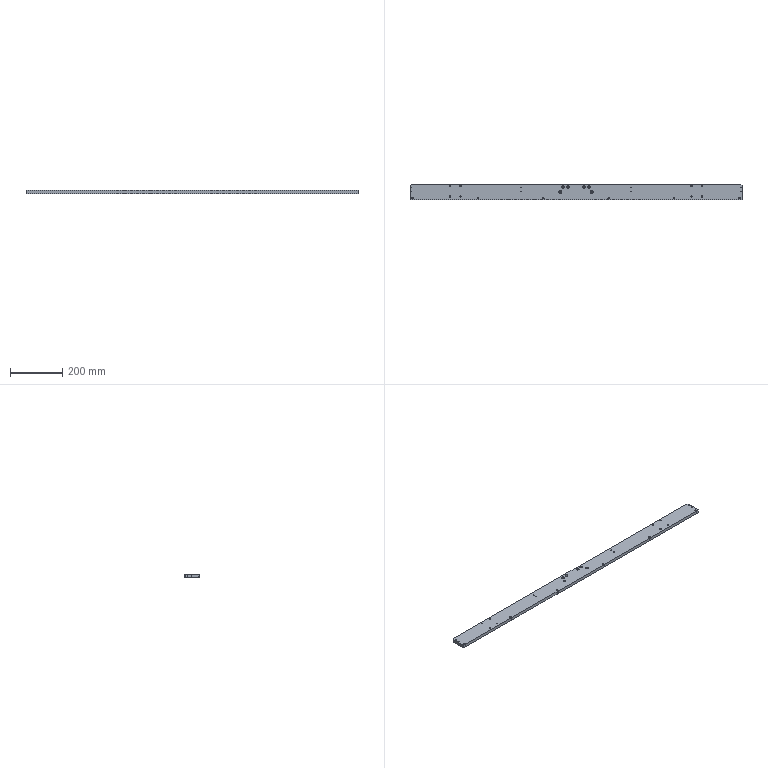Part | SolidWorks | features HoleWzd 4, Chamfer 1, Extrusion 1 | 1 solid | 100 faces | box 1270 x 60 x 12 mm | volume 902865 mm3 | cylinder 80 | plane 20 | commonest cylinder face diameters 3.3 x16 5 x16 5.5 x12 6.6 x12 10 x12 11 x12